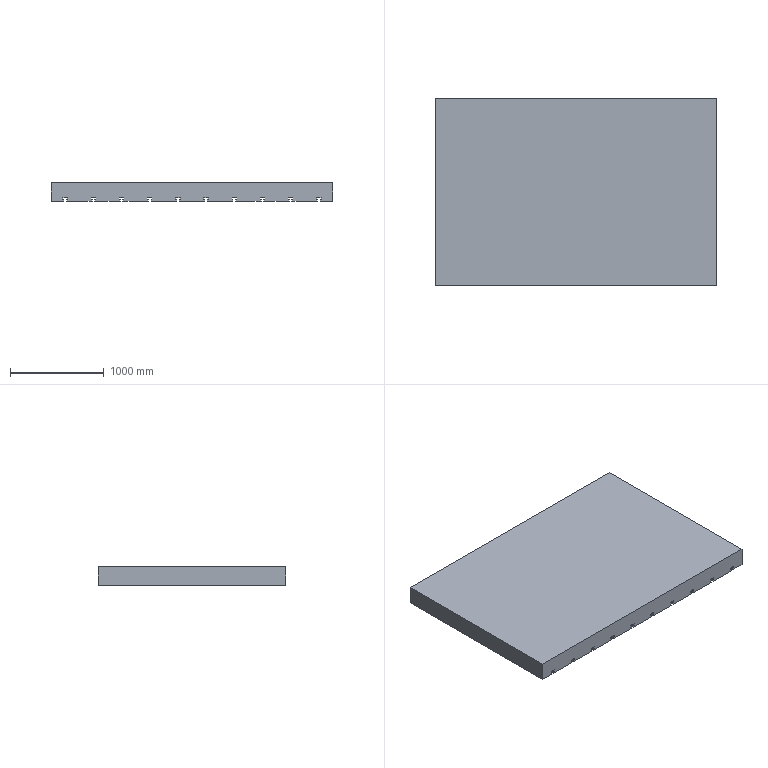Part | NX | features solid 2 | 1 solid | 86 faces | box 3000 x 2000 x 200 mm | volume 1169600000 mm3 | plane 86